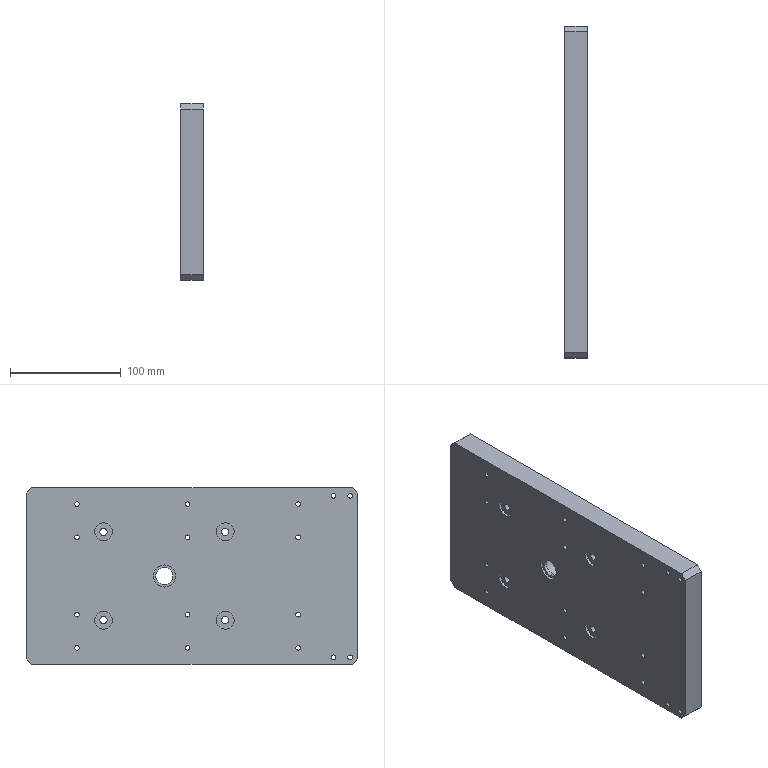Part | SolidWorks | features HoleWzd 5, Chamfer 1, Extrusion 1, ICE 1 | 1 solid | 82 faces | box 20 x 300 x 160 mm | volume 940820 mm3 | cylinder 62 | plane 20 | commonest cylinder face diameters 4.2 x32 6.6 x8 11 x8 16.2 x8 15.5 x2 20 x2